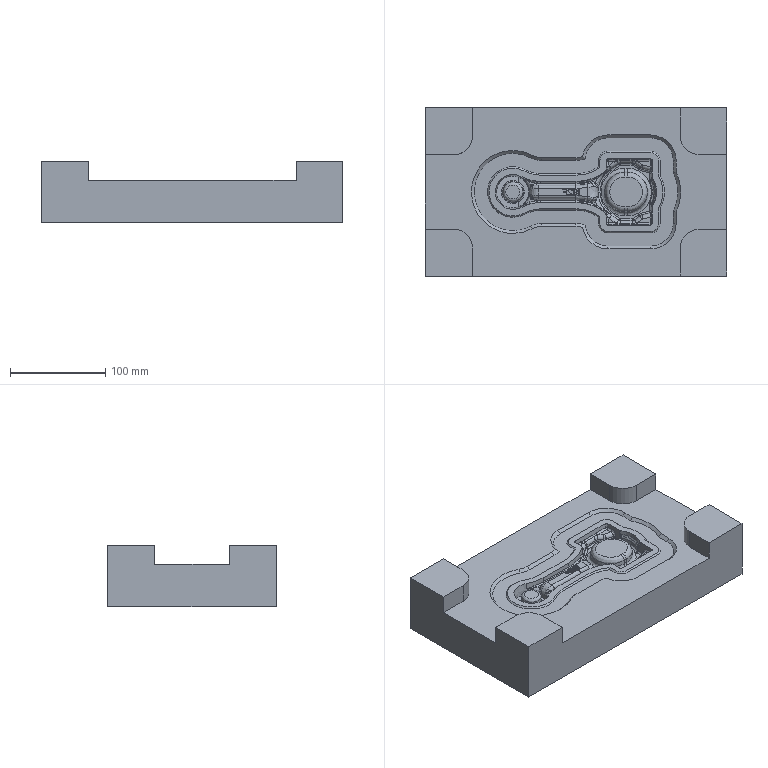NC program | NX | posted with a generic post | part box 317 x 177 x 65 mm
Lines 5565 to 6427 of 8842:
(CAVITY_MILL_COPY_COPY , TOOL : D6)
N11122 M6
N11124 G54
N11126 G17 G0 G90 X48.935 Y-29.973 S3000 M3
N11128 G43 Z10. H0
N11130 Z-21.291
N11132 G94 G1 Z-21.491 F2500.
N11134 G3 X52.726 Y-31.713 R5.
N11136 G1 X77.19
N11138 Y-15.712
N11140 G2 X78.223 Y-12.278 R6.184
N11142 G3 X78.238 Y12.255 R22.119
N11144 G2 X77.19 Y15.684 R6.196
N11146 G1 Y31.713
N11148 X34.853
N11150 Y25.282
N11152 G2 X30.921 Y17.733 R9.221
N11154 X-0.002 Y7.976 R53.878
N11156 G1 X-36.403
N11158 G2 X-59.333 Y13.577 R49.912
N11160 G3 X-59.333 Y-13.577 R-15.315
N11162 G2 X-54.866 Y-11.524 R73.543
N11164 X-36.403 Y-7.976 R50.258
N11166 G1 X-0.002
N11168 G2 X30.92 Y-17.733 R53.878
N11170 X34.853 Y-25.282 R9.221
N11172 G1 Y-31.713
N11174 X52.726
N11176 G3 X56.517 Y-29.973 R5.
N11178 G1 Z-21.291
N11180 G0 Z-19.7
N11182 X48.935 Y-29.939
N11184 Z-21.589
N11186 G1 Z-21.789
N11188 G3 X52.726 Y-31.679 R5.
N11190 G1 X77.164
N11192 Y-15.675
N11194 G2 X78.196 Y-12.271 R6.128
N11196 G3 X78.196 Y12.271 R22.093
N11198 G2 X77.164 Y15.675 R6.128
N11200 G1 Y31.679
N11202 X34.879
N11204 Y25.26
N11206 G2 X30.975 Y17.752 R9.177
N11208 X-0.002 Y7.96 R53.894
N11210 G1 X-36.474
N11212 G2 X-59.358 Y13.549 R49.51
N11214 G3 X-59.358 Y-13.549 R-15.278
N11216 G2 X-36.474 Y-7.96 R49.51
N11218 G1 X-0.002
N11220 G2 X30.974 Y-17.752 R53.894
N11222 X34.879 Y-25.259 R9.176
N11224 G1 Y-31.679
N11226 X52.726
N11228 G3 X56.517 Y-29.939 R5.
N11230 G1 Z-21.589
N11232 G0 Z-21.191
N11234 X48.935 Y-29.905
N11236 Z-21.888
N11238 G1 Z-22.088
N11240 G3 X52.726 Y-31.645 R5.
N11242 G1 X77.138
N11244 Y-15.667
N11246 G2 X78.171 Y-12.262 R6.128
N11248 G3 X78.171 Y12.262 R22.067
N11250 G2 X77.138 Y15.667 R6.128
N11252 G1 Y31.645
N11254 X34.906
N11256 Y25.259
N11258 G2 X31.004 Y17.753 R9.177
N11260 X-0.002 Y7.944 R53.91
N11262 G1 X-36.523
N11264 G2 X-59.383 Y13.52 R49.513
N11266 G3 X-59.383 Y-13.52 R-15.241
N11268 G2 X-36.523 Y-7.944 R49.513
N11270 G1 X-0.002
N11272 G2 X31.004 Y-17.753 R53.91
N11274 X34.906 Y-25.259 R9.176
N11276 G1 Y-31.645
N11278 X52.726
N11280 G3 X56.517 Y-29.905 R5.
N11282 G1 Z-21.888
N11284 G0 Z-21.489
N11286 X48.935 Y-29.871
N11288 Z-22.186
N11290 G1 Z-22.386
N11292 G3 X52.726 Y-31.611 R5.
N11294 G1 X77.112
N11296 Y-15.659
N11298 G2 X78.146 Y-12.253 R6.128
N11300 G3 X78.146 Y12.253 R22.041
N11302 G2 X77.112 Y15.659 R6.128
N11304 G1 Y31.611
N11306 X34.932
N11308 Y25.258
N11310 G2 X31.034 Y17.755 R9.177
N11312 X-0.002 Y7.929 R53.925
N11314 G1 X-36.572
N11316 G2 X-59.408 Y13.492 R49.517
N11318 G3 X-59.408 Y-13.492 R-15.205
N11320 G2 X-36.572 Y-7.929 R49.517
N11322 G1 X-0.002
N11324 G2 X31.034 Y-17.755 R53.925
N11326 X34.932 Y-25.258 R9.177
N11328 G1 Y-31.611
N11330 X52.726
N11332 G3 X56.517 Y-29.871 R5.
N11334 G1 Z-22.186
N11336 G0 Z-21.788
N11338 X48.935 Y-29.837
N11340 Z-22.484
N11342 G1 Z-22.684
N11344 G3 X52.726 Y-31.577 R5.
N11346 G1 X77.086
N11348 Y-15.651
N11350 G2 X78.127 Y-12.234 R6.152
N11352 G3 X78.12 Y12.243 R22.015
N11354 G2 X77.086 Y15.651 R6.128
N11356 G1 Y31.577
N11358 X34.958
N11360 Y25.258
N11362 G2 X31.063 Y17.757 R9.177
N11364 X-0.002 Y7.913 R53.941
N11366 G1 X-36.621
N11368 G2 X-59.433 Y13.464 R49.52
N11370 G3 X-59.433 Y-13.464 R-15.168
N11372 G2 X-36.621 Y-7.913 R49.52
N11374 G1 X-0.002
N11376 G2 X31.063 Y-17.757 R53.941
N11378 X34.958 Y-25.257 R9.177
N11380 G1 Y-31.577
N11382 X52.726
N11384 G3 X56.517 Y-29.837 R5.
N11386 G1 Z-22.484
N11388 G0 Z-20.893
N11390 X-39.386 Y-7.989
N11392 Z-22.484
N11394 G1 Z-22.684
N11396 X-39.392 Y-7.874
N11398 X-39.875 Y-7.812
N11400 X-40.15 Y-7.783
N11402 X-40.475 Y-7.747
N11404 G2 X-44.541 Y-4.191 R4.638
N11406 G3 X-44.569 Y2.932 R35.614
N11408 G2 X-40.759 Y7.72 R4.367
N11410 G1 X-39.875 Y7.829
N11412 X-39.392 Y7.874
N11414 X-0.002
N11416 G3 X12.292 Y9.204 R62.799
N11418 G1 X13.438 Y9.227
N11420 G2 X17.625 Y4.604 R4.132
N11422 G1 X17.534 Y3.842
N11424 G3 X17.7 Y-5.388 R33.723
N11426 G2 X12.292 Y-9.205 R4.608
N11428 G3 X-0.002 Y-7.874 R67.736
N11430 G1 X-39.392
N11432 Z-22.484
N11434 G0 Z-22.086
N11436 X-77.629 Y10.17
N11438 Z-22.484
N11440 G1 X-77.414 Y10.44 Z-22.493
N11442 X-75.439 Y12.187 Z-22.562
N11444 X-74.638 Y12.705 Z-22.587
N11446 X-75.439 Y12.187 Z-22.612
N11448 X-77.414 Y10.44 Z-22.681
N11450 X-79.056 Y8.377 Z-22.75
N11452 X-80.317 Y6.06 Z-22.819
N11454 X-81.156 Y3.561 Z-22.888
N11456 X-81.55 Y0.953 Z-22.957
N11458 Y0. Z-22.982
N11460 G3 X-59.457 Y-13.435 R15.132
N11462 G2 X-41.662 Y-8.153 R49.485
N11464 X-45.681 Y-3.592 R5.047
N11466 G3 X-45.697 Y3.592 R26.053
N11468 G2 X-41.695 Y8.15 R5.048
N11470 X-59.457 Y13.435 R49.699
N11472 G3 X-81.55 Y0. R15.132
N11474 X-76.55 Y-5. R5.
N11476 G1 Z-22.782
N11478 G0 Z-22.384
N11480 X-79.135 Y-8.201
N11482 Z-22.782
N11484 G1 Z-22.982
N11486 X-75.702 Y-5.987
N11488 G2 X-72.406 Y9.283 R11.047
N11490 X-75.702 Y-5.987 R-11.047
N11492 G3 X-77.276 Y-4.898 R2.5
N11494 G1 Z-22.782
N11496 G0 Z-22.384
N11498 X-77.583 Y10.165
N11500 Z-22.782
N11502 G1 X-77.367 Y10.435 Z-22.791
N11504 X-75.388 Y12.178 Z-22.86
N11506 X-74.588 Y12.694 Z-22.885
N11508 X-75.388 Y12.178 Z-22.91
N11510 X-77.367 Y10.435 Z-22.979
N11512 X-79.014 Y8.375 Z-23.048
N11514 X-80.277 Y6.059 Z-23.118
N11516 X-81.119 Y3.56 Z-23.187
N11518 X-81.514 Y0.952 Z-23.256
N11520 Y0. Z-23.281
N11522 G3 X-59.482 Y-13.407 R15.095
N11524 G2 X-42.813 Y-8.26 R49.524
N11526 X-46.401 Y-2.644 R5.103
N11528 G3 X-46.454 Y2.994 R18.566
N11530 G2 X-42.844 Y8.265 R5.18
N11532 X-59.482 Y13.407 R49.439
N11534 G3 X-81.514 Y0. R15.095
N11536 X-79.014 Y-2.5 R2.5
N11538 G1 Z-23.081
N11540 G0 Z-22.384
N11542 X-53.626 Y-4.512
N11544 Z-23.081
N11546 G1 Z-23.281
N11548 G3 X-56.598 Y-6.586 R5.
N11550 G2 X-73.005 Y-9.821 R11.825
N11552 X-56.598 Y-6.586 R-11.825
N11554 G3 X-55.913 Y-10.055 R2.5
N11556 G1 X-54.199 Y-8.3
N11558 Z-23.081
N11560 G0 Z-22.384
N11562 X-77.538 Y10.16
N11564 Z-23.081
N11566 G1 X-77.321 Y10.431 Z-23.09
N11568 X-75.338 Y12.17 Z-23.159
N11570 X-74.537 Y12.683 Z-23.184
N11572 X-75.338 Y12.17 Z-23.209
N11574 X-77.321 Y10.431 Z-23.278
N11576 X-78.971 Y8.372 Z-23.347
N11578 X-80.237 Y6.058 Z-23.416
N11580 X-81.081 Y3.559 Z-23.485
N11582 X-81.477 Y0.951 Z-23.554
N11584 Y0. Z-23.579
N11586 G3 X-59.507 Y-13.378 R15.058
N11588 G2 X-43.663 Y-8.347 R49.585
N11590 X-47.03 Y-2.645 R5.288
N11592 G3 X-47.031 Y2.663 R18.579
N11594 G2 X-43.682 Y8.348 R5.273
N11596 X-59.536 Y13.393 R49.627
N11598 G3 X-81.477 Y0. R15.058
N11600 X-78.977 Y-2.5 R2.5
N11602 G1 Z-23.379
N11604 G0 Z-22.981
N11606 X-79.125 Y-8.081
N11608 Z-23.379
N11610 G1 Z-23.579
N11612 X-76.775 Y-6.586
N11614 G2 X-73.005 Y10.356 R12.273
N11616 X-76.775 Y-6.586 R-12.273
N11618 G3 X-78.341 Y-5.487 R2.5
N11620 G1 Z-23.379
N11622 G0 Z-22.384
N11624 X-54.333 Y-5.068
N11626 Z-23.379
N11628 G3 X-54.333 Y-5.068 Z-23.774 I2.35 J0.489
N11630 X-51.323 Y-6.887 Z-23.877 R2.4
N11632 G2 X-50.01 Y-6.53 R52.507
N11634 X-50.617 Y-2.819 R8.603
N11636 G1 X-50.5 Y-1.895
N11638 G3 X-50.604 Y2.628 R14.493
N11640 G2 X-50.035 Y6.536 R8.473
N11642 X-52.626 Y7.279 R52.525
N11644 X-52.626 Y-7.278 R15.596
N11646 G1 X-55.279 Y-5.878
N11648 G2 X-72.297 Y-11.14 R12.596
N11650 X-55.279 Y-5.878 R-12.596
N11652 G1 X-52.626 Y-7.278
N11654 G2 X-51.323 Y-6.887 R52.507
N11656 G1 X-50.497 Y-9.771
N11658 G2 X-44.337 Y-8.425 R49.507
N11660 X-47.622 Y-2.994 R5.603
N11662 G1 X-47.54 Y-2.395
N11664 X-47.526 Y-2.294
N11666 G3 X-47.623 Y2.994 R17.493
N11668 G2 X-44.33 Y8.424 R5.473
N11670 X-59.56 Y13.365 R49.525
N11672 G3 X-59.531 Y-13.35 R-15.022
N11674 G2 X-50.497 Y-9.771 R49.507
N11676 G3 X-48.782 Y-6.68 R2.5
N11678 G1 Z-23.677
N11680 G0 Z-23.279
N11682 X-47.528 Y-6.317
N11684 Z-23.677
N11686 G3 X-47.528 Y-6.317 Z-24.023 I-2.1 J-0.009
N11688 X-51.593 Y-5.585 Z-24.175 R2.1
N11690 G2 X-52.275 Y-7.139 R15.843
N11692 X-50.464 Y-6.62 R52.551
N11694 X-51.081 Y-3.968 R8.725
N11696 X-51.593 Y-5.585 R15.843
N11698 G1 X-54.4 Y-4.528
N11700 G2 X-54.954 Y5.787 R-12.843
N11702 G1 X-52.275 Y7.139
N11704 G2 X-51.09 Y4.002 R15.843
N11706 X-50.491 Y6.627 R8.571
N11708 X-52.275 Y7.139 R52.699
N11710 G1 X-51.397 Y10.007
N11712 G2 X-59.584 Y13.336 R49.699
N11714 G3 X-59.556 Y-13.321 R-14.985
N11716 G2 X-44.888 Y-8.488 R49.551
N11718 X-48.093 Y-2.994 R5.725
N11720 G1 X-47.991 Y-2.193
N11722 G3 X-48.091 Y2.994 R17.922
N11724 G2 X-44.887 Y8.484 R5.571
N11726 X-51.397 Y10.007 R49.699
N11728 G1 X-52.275 Y7.139
N11730 X-54.954 Y5.787
N11732 G2 X-54.4 Y-4.528 R12.843
N11734 G3 X-52.942 Y-7.748 R2.5
N11736 G1 Z-23.975
N11738 G0 Z-23.577
N11740 X-49.495 Y-7.295
N11742 Z-23.975
N11744 G3 X-49.495 Y-7.295 Z-24.37 I-2.138 J1.09
N11746 X-50.705 Y-3.992 Z-24.474 R2.4
N11748 G1 X-51.633 Y-6.205
N11750 G2 X-52.005 Y-7.026 R16.035
N11752 X-50.884 Y-6.704 R52.639
N11754 X-51.308 Y-5.365 R8.776
N11756 X-51.633 Y-6.205 R16.035
N11758 G1 X-54.4 Y-5.044
N11760 G2 X-54.702 Y5.712 R-13.035
N11762 G1 X-52.005 Y7.026
N11764 G2 X-51.312 Y5.377 R16.035
N11766 X-50.894 Y6.707 R8.71
N11768 X-52.005 Y7.026 R52.588
N11770 G1 X-51.146 Y9.901
N11772 G2 X-59.609 Y13.307 R49.588
N11774 G3 X-59.58 Y-13.293 R-14.949
N11776 G2 X-45.374 Y-8.543 R49.639
N11778 X-48.519 Y-2.994 R5.776
N11780 G3 X-48.475 Y2.64 R19.172
N11782 G2 X-45.373 Y8.544 R5.71
N11784 X-51.146 Y9.901 R49.588
N11786 G1 X-52.005 Y7.026
N11788 X-54.702 Y5.712
N11790 G2 X-54.4 Y-5.044 R13.035
N11792 G3 X-53.062 Y-8.317 R2.5
N11794 G1 Z-24.274
N11796 G0 Z-23.875
N11798 X-49.512 Y-7.699
N11800 Z-24.274
N11802 G3 X-49.512 Y-7.699 Z-24.668 I-2.116 J1.133
N11804 X-50.654 Y-4.372 Z-24.772 R2.4
N11806 G1 X-51.627 Y-6.566
N11808 G2 X-51.796 Y-6.934 R16.183
N11810 X-51.251 Y-6.777 R52.445
N11812 X-51.468 Y-6.193 R8.939
N11814 X-51.627 Y-6.566 R16.183
N11816 G1 X-54.369 Y-5.349
N11818 G2 X-54.507 Y5.649 R-13.183
N11820 G1 X-51.797 Y6.934
N11822 G2 X-51.485 Y6.235 R16.183
N11824 X-51.278 Y6.785 R8.544
N11826 X-51.797 Y6.934 R52.494
N11828 G1 X-50.953 Y9.813
N11830 G2 X-59.633 Y13.278 R49.494
N11832 G3 X-59.605 Y-13.264 R-14.912
N11834 G2 X-45.807 Y-8.599 R49.445
N11836 X-48.912 Y-2.994 R5.939
N11838 G3 X-48.866 Y2.652 R17.422
N11840 G2 X-47.234 Y7.499 R5.544
N11842 G1 X-46.939 Y7.783
N11844 X-45.872 Y8.561
N11846 X-45.808 Y8.599
N11848 G2 X-50.953 Y9.813 R49.494
N11850 G1 X-51.797 Y6.934
N11852 X-54.507 Y5.649
N11854 G2 X-54.369 Y-5.349 R13.183
N11856 G3 X-53.099 Y-8.648 R2.5
N11858 G1 Z-24.572
N11860 G0 Z-24.174
N11862 X-49.525 Y-7.99
N11864 Z-24.572
N11866 G3 X-49.525 Y-7.99 Z-24.967 I-2.099 J1.164
N11868 X-50.618 Y-4.647 Z-25.07 R2.4
N11870 G1 X-51.624 Y-6.826
N11872 X-51.638 Y-6.858
N11874 X-51.589 Y-6.844
N11876 X-51.609 Y-6.795
N11878 X-51.624 Y-6.826
N11880 X-54.348 Y-5.569
N11882 X-54.36 Y-5.595
N11884 G2 X-54.36 Y5.595 R-13.294
N11886 G1 X-51.638 Y6.858
N11888 X-51.605 Y6.785
N11890 X-51.581 Y6.842
N11892 X-51.638 Y6.858
N11894 X-50.806 Y9.74
N11896 G2 X-59.657 Y13.25 R49.474
N11898 G3 X-59.629 Y-13.236 R-14.875
N11900 G2 X-46.171 Y-8.642 R49.324
N11902 X-49.197 Y-2.577 R5.91
N11904 G3 X-49.25 Y2.994 R17.765
N11906 G2 X-46.178 Y8.642 R5.984
N11908 X-50.806 Y9.74 R49.474
N11910 G1 X-51.638 Y6.858
N11912 X-54.36 Y5.595
N11914 G2 X-54.336 Y-5.544 R13.294
N11916 G1 X-54.348 Y-5.569
N11918 G3 X-53.125 Y-8.887 R2.5
N11920 G1 Z-24.87
N11922 G0 Z-22.384
N11924 X-77.261 Y10.129
N11926 Z-24.87
N11928 G1 X-76.977 Y10.47 Z-24.882
N11930 X-75.035 Y12.118 Z-24.948
N11932 X-74.232 Y12.615 Z-24.973
N11934 X-75.035 Y12.118 Z-24.998
N11936 X-76.977 Y10.47 Z-25.064
N11938 X-78.608 Y8.514 Z-25.131
N11940 X-79.883 Y6.309 Z-25.198
N11942 X-80.762 Y3.919 Z-25.265
N11944 X-81.22 Y1.414 Z-25.331
N11946 X-81.257 Y0.235 Z-25.362
N11948 Y0. Z-25.368
N11950 G3 X-59.68 Y-13.22 R14.839
N11952 G2 X-46.526 Y-8.685 R49.337
N11954 X-49.5 Y-2.395 R6.053
N11956 G3 X-49.509 Y2.443 R15.558
N11958 G2 X-46.527 Y8.682 R6.09
N11960 X-59.68 Y13.22 R49.572
N11962 G3 X-81.257 Y0. R14.839
N11964 X-80.525 Y-1.768 R2.5
N11966 G1 Z-25.168
N11968 G0 Z-24.77
N11970 X-78.934 Y-7.973
N11972 Z-25.168
N11974 G1 Z-25.368
N11976 X-77.696 Y-7.185
N11978 G2 X-73.603 Y11.278 R13.372
N11980 X-77.696 Y-7.185 R-13.372
N11982 G3 X-79.264 Y-6.087 R2.5
N11984 G1 Z-25.168
N11986 G0 Z-22.981
N11988 X-77.219 Y10.126
N11990 Z-25.168
N11992 G1 X-76.996 Y10.398 Z-25.177
N11994 X-74.984 Y12.109 Z-25.247
N11996 X-74.181 Y12.603 Z-25.271
N11998 X-74.984 Y12.109 Z-25.296
N12000 X-76.996 Y10.398 Z-25.365
N12002 X-78.673 Y8.357 Z-25.434
N12004 X-79.96 Y6.051 Z-25.503
N12006 X-80.819 Y3.553 Z-25.573
N12008 X-81.221 Y0.943 Z-25.642
N12010 Y0. Z-25.666
N12012 G3 X-59.704 Y-13.191 R14.802
N12014 G2 X-46.846 Y-8.72 R49.469
N12016 X-49.74 Y-4.79 R6.566
N12018 X-49.785 Y-2.395 R6.784
N12020 G3 X-49.784 Y2.395 R16.324
N12022 G2 X-46.824 Y8.718 R6.15
N12024 X-59.704 Y13.191 R49.365
N12026 G3 X-81.221 Y0. R14.802
N12028 X-80.489 Y-1.768 R2.5
N12030 G1 Z-25.466
N12032 G0 Z-25.068
N12034 X-78.921 Y-7.925
N12036 Z-25.466
N12038 G1 Z-25.666
N12040 X-77.752 Y-7.185
N12042 G2 X-73.603 Y11.333 R13.419
N12044 X-77.752 Y-7.185 R-13.419
N12046 G3 X-79.317 Y-6.084 R2.5
N12048 G1 Z-25.466
N12050 G0 Z-22.981
N12052 X-77.173 Y10.121
N12054 Z-25.466
N12056 G1 X-76.949 Y10.393 Z-25.476
N12058 X-74.933 Y12.1 Z-25.545
N12060 X-74.13 Y12.592 Z-25.57
N12062 X-74.933 Y12.1 Z-25.594
N12064 X-76.949 Y10.393 Z-25.663
N12066 X-78.63 Y8.354 Z-25.733
N12068 X-79.921 Y6.05 Z-25.802
N12070 X-80.781 Y3.552 Z-25.871
N12072 X-81.184 Y0.942 Z-25.94
N12074 Y0. Z-25.965
N12076 G3 X-59.746 Y-13.172 R14.765
N12078 G2 X-47.122 Y-8.748 R49.549
N12080 X-50.07 Y-2.395 R6.362
N12082 G3 X-50.07 Y2.395 R14.499
N12084 G2 X-47.114 Y8.754 R6.344
N12086 X-59.719 Y13.158 R49.174
N12088 G3 X-81.184 Y0. R14.765
N12090 X-80.452 Y-1.768 R2.5
N12092 G1 Z-25.765
N12094 G0 Z-25.366
N12096 X-78.9 Y-7.89
N12098 Z-25.765
N12100 G1 Z-25.965
N12102 X-77.784 Y-7.185
N12104 G2 X-73.603 Y11.365 R13.446
N12106 X-77.784 Y-7.185 R-13.446
N12108 G3 X-79.347 Y-6.082 R2.5
N12110 G1 Z-25.765
N12112 G0 Z-22.981
N12114 X-77.128 Y10.116
N12116 Z-25.765
N12118 G1 X-76.903 Y10.388 Z-25.774
N12120 X-74.883 Y12.091 Z-25.843
N12122 X-74.079 Y12.58 Z-25.868
N12124 X-74.883 Y12.091 Z-25.892
N12126 X-76.903 Y10.388 Z-25.962
N12128 X-78.587 Y8.352 Z-26.031
N12130 X-79.881 Y6.049 Z-26.1
N12132 X-80.744 Y3.552 Z-26.169
N12134 X-81.148 Y0.941 Z-26.238
N12136 Y0. Z-26.263
N12138 G3 X-59.79 Y-13.153 R14.729
N12140 G2 X-47.376 Y-8.775 R49.504
N12142 X-50.045 Y-5.388 R6.929
N12144 X-50.328 Y-2.536 R5.741
N12146 G3 X-50.316 Y2.45 R16.568
N12148 G2 X-48.618 Y7.707 R6.209
N12150 G1 X-48.399 Y7.932
N12152 G2 X-47.372 Y8.78 R6.271
N12154 X-59.727 Y13.121 R49.039
N12156 G3 X-81.148 Y0. R14.729
N12158 X-80.415 Y-1.768 R2.5
N12160 G1 Z-26.063
N12162 G0 Z-25.665
N12164 X-78.878 Y-7.855
N12166 Z-26.063
N12168 G1 Z-26.263
N12170 X-77.815 Y-7.185
N12172 G2 X-73.603 Y11.396 R13.472
N12174 X-77.815 Y-7.185 R-13.472
N12176 G3 X-79.377 Y-6.08 R2.5
N12178 G1 Z-26.063
N12180 G0 Z-22.981
N12182 X-77.082 Y10.111
N12184 Z-26.063
N12186 G1 X-76.856 Y10.383 Z-26.072
N12188 X-74.832 Y12.082 Z-26.141
N12190 X-74.028 Y12.568 Z-26.166
N12192 X-74.832 Y12.082 Z-26.191
N12194 X-76.856 Y10.383 Z-26.26
N12196 X-78.544 Y8.35 Z-26.329
N12198 X-79.841 Y6.048 Z-26.398
N12200 X-80.706 Y3.551 Z-26.467
N12202 X-81.111 Y0.939 Z-26.537
N12204 Y0. Z-26.561
N12206 G3 X-59.751 Y-13.092 R14.692
N12208 G2 X-47.588 Y-8.787 R49.529
N12210 X-50.608 Y-2.994 R6.675
N12212 G3 X-50.45 Y1.796 R20.661
N12214 G1 X-50.546 Y2.395
N12216 G2 X-47.585 Y8.789 R6.611
N12218 X-59.751 Y13.092 R49.424
N12220 G3 X-81.111 Y0. R14.692
N12222 X-80.379 Y-1.768 R2.5
N12224 G1 Z-26.361
N12226 G0 Z-25.963
N12228 X-78.857 Y-7.82
N12230 Z-26.361
N12232 G1 Z-26.561
N12234 X-77.846 Y-7.185
N12236 G2 X-73.603 Y11.427 R13.498
N12238 X-77.846 Y-7.185 R-13.498
N12240 G3 X-79.406 Y-6.078 R2.5
N12242 G1 Z-26.361
N12244 G0 Z-22.981
N12246 X-77.036 Y10.106
N12248 Z-26.361
N12250 G1 X-76.809 Y10.378 Z-26.37
N12252 X-74.781 Y12.072 Z-26.44
N12254 X-73.977 Y12.556 Z-26.464
N12256 X-74.781 Y12.072 Z-26.489
N12258 X-76.809 Y10.378 Z-26.558
N12260 X-78.501 Y8.347 Z-26.627
N12262 X-79.802 Y6.047 Z-26.696
N12264 X-80.669 Y3.55 Z-26.766
N12266 X-81.074 Y0.938 Z-26.835
N12268 Y0. Z-26.859
N12270 G3 X-59.773 Y-13.062 R14.656
N12272 G2 X-47.883 Y-8.753 R53.364
N12274 G1 X-48.27 Y-8.446
N12276 G2 X-50.756 Y-2.395 R6.693
N12278 G1 X-50.68 Y-1.796
N12280 G3 X-50.739 Y2.263 R16.022
N12282 G2 X-47.855 Y8.751 R6.686
N12284 X-52.468 Y10.054 R39.01
N12286 X-59.776 Y13.063 R51.451
N12288 G3 X-81.074 Y0. R14.656
N12290 X-80.342 Y-1.768 R2.5
N12292 G1 Z-26.659
N12294 G0 Z-26.261
N12296 X-78.835 Y-7.786
N12298 Z-26.659
N12300 G1 Z-26.859
N12302 X-77.876 Y-7.185
N12304 G2 X-73.603 Y11.458 R13.524
N12306 X-77.876 Y-7.185 R-13.524
N12308 G3 X-79.436 Y-6.076 R2.5
N12310 G1 Z-26.659
N12312 G0 Z-22.981
N12314 X-76.99 Y10.101
N12316 Z-26.659
N12318 G1 X-76.763 Y10.373 Z-26.669
N12320 X-74.73 Y12.063 Z-26.738
N12322 X-73.926 Y12.544 Z-26.762
N12324 X-74.73 Y12.063 Z-26.787
N12326 X-76.763 Y10.373 Z-26.856
N12328 X-78.458 Y8.345 Z-26.925
N12330 X-79.762 Y6.046 Z-26.995
N12332 X-80.631 Y3.549 Z-27.064
N12334 X-81.038 Y0.937 Z-27.133
N12336 Y0. Z-27.158
N12338 G3 X-59.764 Y-13.016 R14.619
N12340 G2 X-52.974 Y-10.178 R52.685
N12342 X-48.24 Y-8.68 R26.728
N12344 X-50.944 Y-2.395 R7.008
N12346 G3 X-51.011 Y2.994 R19.33
N12348 G2 X-48.234 Y8.679 R7.103
N12350 X-52.468 Y9.99 R22.84
N12352 X-59.775 Y13.022 R57.838
N12354 G3 X-81.038 Y0. R14.619
N12356 X-80.306 Y-1.768 R2.5
N12358 G1 Z-26.958
N12360 G0 Z-26.559
N12362 X-78.814 Y-7.751
N12364 Z-26.958
N12366 G1 Z-27.158
N12368 X-77.907 Y-7.185
N12370 G2 X-73.603 Y11.488 R13.55
N12372 X-77.907 Y-7.185 R-13.55
N12374 G3 X-79.465 Y-6.074 R2.5
N12376 G1 Z-26.958
N12378 G0 Z-22.981
N12380 X-76.944 Y10.095
N12382 Z-26.958
N12384 G1 X-76.716 Y10.368 Z-26.967
N12386 X-74.679 Y12.054 Z-27.036
N12388 X-73.875 Y12.532 Z-27.061
N12390 X-74.679 Y12.054 Z-27.085
N12392 X-76.716 Y10.368 Z-27.154
N12394 X-78.415 Y8.343 Z-27.224
N12396 X-79.722 Y6.044 Z-27.293
N12398 X-80.594 Y3.548 Z-27.362
N12400 X-81.001 Y0.936 Z-27.431
N12402 Y0. Z-27.456
N12404 G3 X-59.755 Y-12.971 R14.582
N12406 G2 X-53.667 Y-10.364 R58.835
N12408 G1 X-51.268 Y-9.289
N12410 G2 X-48.854 Y-8.535 R10.435
N12412 X-51.16 Y-3.592 R8.234
N12414 X-51.092 Y-2.002 R10.516
N12416 G3 X-51.137 Y2.395 R17.147
N12418 G2 X-50.534 Y5.987 R6.814
N12420 X-48.856 Y8.532 R7.331
N12422 X-51.386 Y9.335 R10.968
N12424 G1 X-52.468 Y9.829
N12426 G3 X-56.046 Y11.288 R217.569
N12428 G2 X-59.766 Y12.976 R42.827
N12430 G3 X-81.001 Y0. R14.582
N12432 X-80.269 Y-1.768 R2.5
N12434 G1 Z-27.256
N12436 G0 Z-26.858
N12438 X-78.792 Y-7.717
N12440 Z-27.256
N12442 G1 Z-27.456
N12444 X-77.938 Y-7.185
N12446 G2 X-73.603 Y11.519 R13.576
N12448 X-77.938 Y-7.185 R-13.576
N12450 G3 X-79.495 Y-6.072 R2.5
N12452 G1 Z-27.256
N12454 G0 Z-22.981
N12456 X-76.887 Y10.087
N12458 Z-27.256
N12460 G1 X-76.351 Y10.668 Z-27.277
N12462 X-74.628 Y12.044 Z-27.334
N12464 X-73.824 Y12.52 Z-27.359
N12466 X-74.628 Y12.044 Z-27.383
N12468 X-76.351 Y10.668 Z-27.441
N12470 X-77.846 Y9.048 Z-27.499
N12472 X-79.08 Y7.222 Z-27.556
N12474 X-80.025 Y5.229 Z-27.614
N12476 X-80.658 Y3.118 Z-27.672
N12478 X-80.965 Y0.935 Z-27.73
N12480 Y0. Z-27.754
N12482 G3 X-59.746 Y-12.925 R14.546
N12484 G2 X-55.212 Y-10.923 R50.5
N12486 G3 X-51.268 Y-8.656 R14.74
N12488 G1 X-50.079 Y-8.024
N12490 X-50.202 Y-7.783
N12492 X-51.1 Y-4.79
N12494 X-51.172 Y-4.49
N12496 G2 X-51.282 Y-2.145 R6.278
N12498 G3 X-51.271 Y2.088 R15.312
N12500 G2 X-50.998 Y5.173 R6.956
N12502 G1 X-50.07 Y8.042
N12504 X-50.669 Y8.325
N12506 X-52.894 Y9.779
N12508 G3 X-54.735 Y10.629 R28.791
N12510 G2 X-59.757 Y12.931 R85.718
N12512 G3 X-80.965 Y0. R14.546
N12514 X-80.233 Y-1.768 R2.5
N12516 G1 Z-27.554
N12518 G0 Z-27.156
N12520 X-78.77 Y-7.683
N12522 Z-27.554
N12524 G1 Z-27.754
N12526 X-77.968 Y-7.185
N12528 G2 X-73.603 Y11.55 R13.602
N12530 X-77.968 Y-7.185 R-13.602
N12532 G3 X-79.524 Y-6.07 R2.5
N12534 G1 Z-27.554
N12536 G0 Z-22.981
N12538 X-76.841 Y10.082
N12540 Z-27.554
N12542 G1 X-76.303 Y10.663 Z-27.575
N12544 X-74.577 Y12.035 Z-27.633
N12546 X-73.772 Y12.508 Z-27.657
N12548 X-74.577 Y12.035 Z-27.681
N12550 X-76.303 Y10.663 Z-27.739
N12552 X-77.802 Y9.045 Z-27.797
N12554 X-79.039 Y7.22 Z-27.855
N12556 X-79.985 Y5.229 Z-27.912
N12558 X-80.62 Y3.117 Z-27.97
N12560 X-80.928 Y0.934 Z-28.028
N12562 Y0. Z-28.052
N12564 G3 X-59.738 Y-12.879 R14.509
N12566 G2 X-53.85 Y-9.998 R161.051
N12568 G3 X-51.179 Y-5.126 R15.187
N12570 G2 X-51.421 Y-2.075 R7.469
N12572 G3 X-51.422 Y2.055 R16.312
N12574 G2 X-51.182 Y5.104 R7.494
N12576 G3 X-53.883 Y9.946 R13.183
N12578 G2 X-59.703 Y12.861 R383.797
N12580 G3 X-80.928 Y0. R14.509
N12582 X-80.196 Y-1.768 R2.5
N12584 G1 Z-27.852
N12586 G0 Z-27.454
N12588 X-78.748 Y-7.649
N12590 Z-27.852
N12592 G1 Z-28.052
N12594 X-77.999 Y-7.185
N12596 G2 X-73.603 Y11.581 R13.628
N12598 X-77.999 Y-7.185 R-13.628
N12600 G3 X-79.554 Y-6.068 R2.5
N12602 G1 Z-27.852
N12604 G0 Z-22.981
N12606 X-76.795 Y10.077
N12608 Z-27.852
N12610 G1 X-76.255 Y10.657 Z-27.873
N12612 X-74.526 Y12.025 Z-27.931
N12614 X-73.721 Y12.495 Z-27.955
N12616 X-74.526 Y12.025 Z-27.98
N12618 X-76.255 Y10.657 Z-28.037
N12620 X-77.757 Y9.042 Z-28.095
N12622 X-78.997 Y7.218 Z-28.153
N12624 X-79.946 Y5.228 Z-28.211
N12626 X-80.583 Y3.116 Z-28.268
N12628 X-80.891 Y0.932 Z-28.326
N12630 Y0. Z-28.351
N12632 G3 X-59.254 Y-12.575 R14.472
N12634 G1 X-58.464 Y-12.122
N12636 X-54.866 Y-10.122
N12638 X-54.394 Y-9.864
N12640 G3 X-51.484 Y-4.346 R14.819
N12642 G2 X-51.548 Y-1.796 R7.763
N12644 G3 X-51.548 Y1.796 R13.258
N12646 G2 X-51.481 Y4.365 R7.624
N12648 G3 X-54.534 Y9.935 R13.703
N12650 G1 X-59.492 Y12.707
N12652 G3 X-80.891 Y0. R14.472
N12654 X-80.159 Y-1.768 R2.5
N12656 G1 Z-28.151
N12658 G0 Z-27.752
N12660 X-78.726 Y-7.615
N12662 Z-28.151
N12664 G1 Z-28.351
N12666 X-78.03 Y-7.185
N12668 G2 X-73.603 Y11.611 R13.654
N12670 X-78.03 Y-7.185 R-13.654
N12672 G1 Z-28.151
N12674 G0 Z-22.682
N12676 X-76.749 Y10.071
N12678 Z-28.151
N12680 G1 X-76.208 Y10.651 Z-28.171
N12682 X-74.474 Y12.015 Z-28.229
N12684 X-73.669 Y12.483 Z-28.253
N12686 X-74.474 Y12.015 Z-28.278
N12688 X-76.208 Y10.651 Z-28.336
N12690 X-77.713 Y9.039 Z-28.393
N12692 X-78.956 Y7.217 Z-28.451
N12694 X-79.907 Y5.227 Z-28.509
N12696 X-80.545 Y3.115 Z-28.567
N12698 X-80.855 Y0.931 Z-28.624
N12700 Y0. Z-28.649
N12702 G3 X-58.806 Y-12.266 R14.436
N12704 X-54.75 Y-9.752 R371.857
N12706 X-51.693 Y-3.794 R14.766
N12708 G2 X-51.677 Y-1.796 R7.772
N12710 G3 X-51.677 Y1.796 R14.472
N12712 G2 X-51.7 Y3.769 R8.348
N12714 G3 X-54.728 Y9.687 R14.275
N12716 G1 X-55.138 Y10.006
N12718 X-57.265 Y11.323
N12720 X-57.355 Y11.375
N12722 X-59.064 Y12.422
N12724 G3 X-80.855 Y0. R14.436
N12726 X-80.122 Y-1.768 R2.5
N12728 G1 Z-28.449
N12730 G0 Z-28.051
N12732 X-78.704 Y-7.581
N12734 Z-28.449
N12736 G1 Z-28.649
N12738 X-78.061 Y-7.185
N12740 G2 X-73.603 Y11.642 R13.68
N12742 X-78.061 Y-7.185 R-13.68
N12744 G1 Z-28.449
N12746 G0 Z-22.682
N12748 X-76.703 Y10.066
N12750 Z-28.449
N12752 G1 X-76.16 Y10.645 Z-28.47
N12754 X-74.423 Y12.006 Z-28.527
N12756 X-73.618 Y12.471 Z-28.552
N12758 X-74.423 Y12.006 Z-28.576
N12760 X-76.16 Y10.645 Z-28.634
N12762 X-77.669 Y9.036 Z-28.692
N12764 X-78.915 Y7.215 Z-28.749
N12766 X-79.869 Y5.226 Z-28.807
N12768 X-80.508 Y3.114 Z-28.865
N12770 X-80.818 Y0.93 Z-28.923
N12772 Y0. Z-28.947
N12774 G3 X-58.422 Y-11.975 R14.399
N12776 G1 X-57.864 Y-11.603
N12778 X-55.466 Y-9.967
N12780 X-55.186 Y-9.804
N12782 G3 X-52.273 Y-4.79 R13.648
N12784 G1 X-52.075 Y-4.191
N12786 G3 X-51.864 Y-2.395 R4.097
N12788 X-51.737 Y1.197 R16.268
N12790 G1 X-51.803 Y1.796
N12792 G2 X-51.868 Y3.334 R10.108
N12794 G3 X-54.558 Y9.068 R14.771
N12796 X-55.613 Y10.078 R4.797
N12798 X-58.422 Y11.974 R101.848
N12800 X-80.818 Y0. R14.399
N12802 X-80.086 Y-1.768 R2.5
N12804 G1 Z-28.747
N12806 G0 Z-28.349
N12808 X-78.681 Y-7.548
N12810 Z-28.747
N12812 G1 Z-28.947
N12814 X-78.091 Y-7.185
N12816 G2 X-73.603 Y11.673 R13.706
N12818 X-78.091 Y-7.185 R-13.706
N12820 G1 Z-28.747
N12822 G0 Z-22.384
N12824 X-76.657 Y10.06
N12826 Z-28.747
N12828 G1 X-76.112 Y10.639 Z-28.768
N12830 X-74.372 Y11.996 Z-28.826
N12832 X-73.566 Y12.458 Z-28.85
N12834 X-74.372 Y11.996 Z-28.874
N12836 X-76.112 Y10.639 Z-28.932
N12838 X-77.624 Y9.032 Z-28.99
N12840 X-78.873 Y7.213 Z-29.048